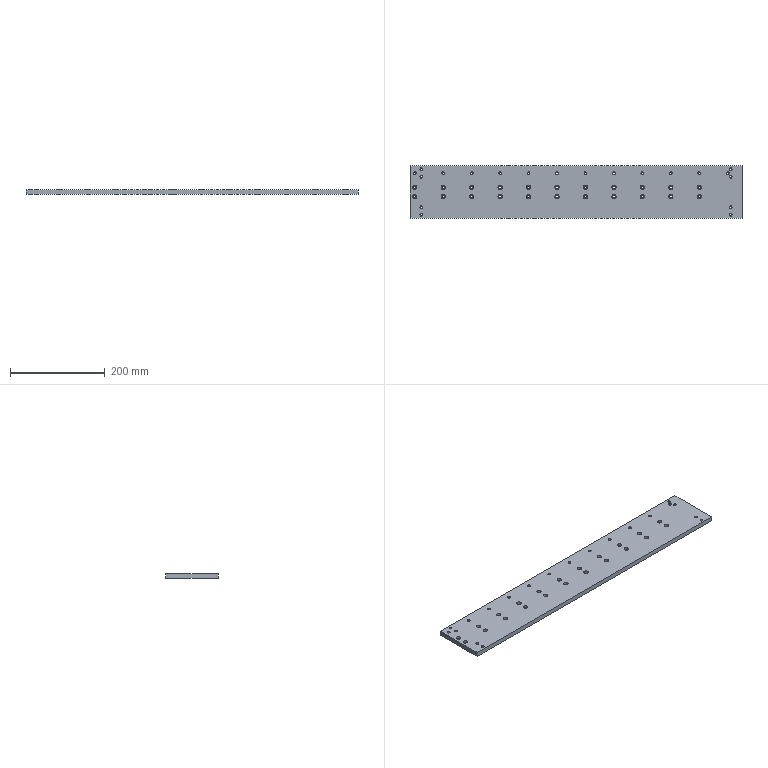Part | NX | features CBORE_HOLE 22, SIMPLE HOLE 20, SYMBOLIC_THREAD 20, DATUM_CSYS 15, SKETCH 14, HOLE PACKAGE 13, EXTRACT_DATUM_PLANE 11, EXTRACT_FACE 11, Instance Feature 10, EXTRUDE 1, Pattern Feature 1 | 1 solid | 132 faces | box 700 x 110 x 10 mm | volume 755648 mm3 | cylinder 64 | cone 40 | plane 28 | commonest cylinder face diameters 5.5 x22 9 x22 5.2 x20